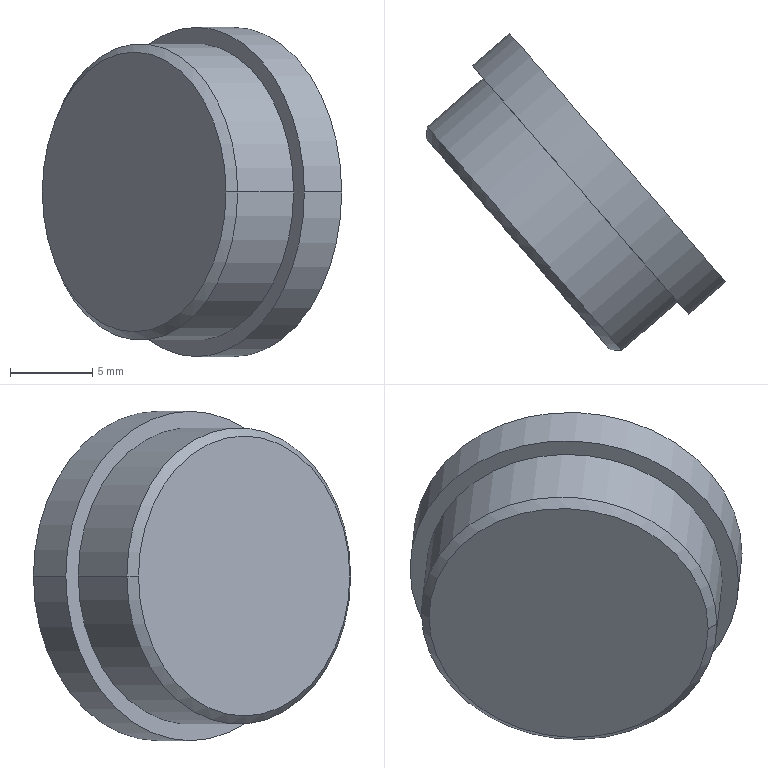Part | SolidWorks | features Chamfer 1, Revolution 1 | 1 solid | 9 faces | box 18.175 x 19.26 x 20 mm | volume 2208 mm3 | cylinder 4 | plane 3 | cone 2 | commonest cylinder face diameters 18 x2 20 x2
STEP:
#1=CARTESIAN_POINT('',(1439.201,-61.47,0.));
#2=VERTEX_POINT('',#1);
#3=CARTESIAN_POINT('',(1428.048,-48.64,0.));
#4=VERTEX_POINT('',#3);
#5=CARTESIAN_POINT('',(1433.624,-55.055,0.));
#6=DIRECTION('',(-0.7547,-0.6561,0.));
#7=DIRECTION('',(0.6561,-0.7547,0.));
#8=AXIS2_PLACEMENT_3D('',#5,#6,#7);
#9=CIRCLE('',#8,8.5);
#10=EDGE_CURVE('',#2,#4,#9,.T.);
#11=ORIENTED_EDGE('',*,*,#10,.F.);
#12=CARTESIAN_POINT('',(1439.906,-61.519,0.));
#13=VERTEX_POINT('',#12);
#14=CARTESIAN_POINT('',(1439.906,-61.519,0.));
#15=DIRECTION('',(0.9976,-0.06976,0.));
#16=VECTOR('',#15,1000.);
#17=LINE('',#14,#16);
#18=EDGE_CURVE('',#2,#13,#17,.T.);
#19=ORIENTED_EDGE('',*,*,#18,.T.);
#20=CARTESIAN_POINT('',(1428.097,-47.934,0.));
#21=VERTEX_POINT('',#20);
#22=CARTESIAN_POINT('',(1434.002,-54.727,0.));
#23=DIRECTION('',(0.7547,0.6561,0.));
#24=DIRECTION('',(0.6561,-0.7547,0.));
#25=AXIS2_PLACEMENT_3D('',#22,#23,#24);
#26=CIRCLE('',#25,9.);
#27=EDGE_CURVE('',#21,#13,#26,.T.);
#28=ORIENTED_EDGE('',*,*,#27,.F.);
#29=CARTESIAN_POINT('',(1428.097,-47.934,0.));
#30=DIRECTION('',(0.06976,0.9976,0.));
#31=VECTOR('',#30,1000.);
#32=LINE('',#29,#31);
#33=EDGE_CURVE('',#4,#21,#32,.T.);
#34=ORIENTED_EDGE('',*,*,#33,.F.);
#35=EDGE_LOOP('',(#11,#19,#28,#34));
#36=FACE_OUTER_BOUND('',#35,.T.);
#37=CARTESIAN_POINT('',(1434.002,-54.727,0.));
#38=DIRECTION('',(0.7547,0.6561,0.));
#39=DIRECTION('',(-0.6561,0.7547,0.));
#40=AXIS2_PLACEMENT_3D('',#37,#38,#39);
#41=CONICAL_SURFACE('',#40,9.,0.7854);
#42=ADVANCED_FACE('',(#36),#41,.T.);
#43=CARTESIAN_POINT('',(1430.837,-44.227,0.));
#44=VERTEX_POINT('',#43);
#45=CARTESIAN_POINT('',(1443.958,-59.322,0.));
#46=VERTEX_POINT('',#45);
#47=CARTESIAN_POINT('',(1437.398,-51.775,0.));
#48=DIRECTION('',(0.7547,0.6561,0.));
#49=DIRECTION('',(-0.6561,0.7547,0.));
#50=AXIS2_PLACEMENT_3D('',#47,#48,#49);
#51=CIRCLE('',#50,10.);
#52=EDGE_CURVE('',#44,#46,#51,.T.);
#53=ORIENTED_EDGE('',*,*,#52,.T.);
#54=CARTESIAN_POINT('',(1446.223,-57.354,0.));
#55=VERTEX_POINT('',#54);
#56=CARTESIAN_POINT('',(1446.223,-57.354,0.));
#57=DIRECTION('',(0.7547,0.6561,0.));
#58=VECTOR('',#57,1000.);
#59=LINE('',#56,#58);
#60=EDGE_CURVE('',#46,#55,#59,.T.);
#61=ORIENTED_EDGE('',*,*,#60,.T.);
#62=CARTESIAN_POINT('',(1433.101,-42.259,0.));
#63=VERTEX_POINT('',#62);
#64=CARTESIAN_POINT('',(1439.662,-49.806,0.));
#65=DIRECTION('',(0.7547,0.6561,0.));
#66=DIRECTION('',(-0.6561,0.7547,0.));
#67=AXIS2_PLACEMENT_3D('',#64,#65,#66);
#68=CIRCLE('',#67,10.);
#69=EDGE_CURVE('',#63,#55,#68,.T.);
#70=ORIENTED_EDGE('',*,*,#69,.F.);
#71=CARTESIAN_POINT('',(1433.101,-42.259,0.));
#72=DIRECTION('',(0.7547,0.6561,0.));
#73=VECTOR('',#72,1000.);
#74=LINE('',#71,#73);
#75=EDGE_CURVE('',#44,#63,#74,.T.);
#76=ORIENTED_EDGE('',*,*,#75,.F.);
#77=EDGE_LOOP('',(#53,#61,#70,#76));
#78=FACE_OUTER_BOUND('',#77,.T.);
#79=CARTESIAN_POINT('',(1439.662,-49.806,0.));
#80=DIRECTION('',(0.7547,0.6561,0.));
#81=DIRECTION('',(-0.6561,0.7547,0.));
#82=AXIS2_PLACEMENT_3D('',#79,#80,#81);
#83=CYLINDRICAL_SURFACE('',#82,10.);
#84=ADVANCED_FACE('',(#78),#83,.T.);
#85=ORIENTED_EDGE('',*,*,#27,.T.);
#86=CARTESIAN_POINT('',(1443.302,-58.567,0.));
#87=VERTEX_POINT('',#86);
#88=CARTESIAN_POINT('',(1445.566,-56.599,0.));
#89=DIRECTION('',(0.7547,0.6561,0.));
#90=VECTOR('',#89,1000.);
#91=LINE('',#88,#90);
#92=EDGE_CURVE('',#13,#87,#91,.T.);
#93=ORIENTED_EDGE('',*,*,#92,.T.);
#94=CARTESIAN_POINT('',(1431.493,-44.982,0.));
#95=VERTEX_POINT('',#94);
#96=CARTESIAN_POINT('',(1437.398,-51.775,0.));
#97=DIRECTION('',(0.7547,0.6561,0.));
#98=DIRECTION('',(-0.6561,0.7547,0.));
#99=AXIS2_PLACEMENT_3D('',#96,#97,#98);
#100=CIRCLE('',#99,9.);
#101=EDGE_CURVE('',#95,#87,#100,.T.);
#102=ORIENTED_EDGE('',*,*,#101,.F.);
#103=CARTESIAN_POINT('',(1433.757,-43.014,0.));
#104=DIRECTION('',(0.7547,0.6561,0.));
#105=VECTOR('',#104,1000.);
#106=LINE('',#103,#105);
#107=EDGE_CURVE('',#21,#95,#106,.T.);
#108=ORIENTED_EDGE('',*,*,#107,.F.);
#109=EDGE_LOOP('',(#85,#93,#102,#108));
#110=FACE_OUTER_BOUND('',#109,.T.);
#111=CARTESIAN_POINT('',(1439.662,-49.806,0.));
#112=DIRECTION('',(0.7547,0.6561,0.));
#113=DIRECTION('',(-0.6561,0.7547,0.));
#114=AXIS2_PLACEMENT_3D('',#111,#112,#113);
#115=CYLINDRICAL_SURFACE('',#114,9.);
#116=ADVANCED_FACE('',(#110),#115,.T.);
#117=ORIENTED_EDGE('',*,*,#92,.F.);
#118=CARTESIAN_POINT('',(1434.002,-54.727,0.));
#119=DIRECTION('',(0.7547,0.6561,0.));
#120=DIRECTION('',(0.6561,-0.7547,0.));
#121=AXIS2_PLACEMENT_3D('',#118,#119,#120);
#122=CIRCLE('',#121,9.);
#123=EDGE_CURVE('',#13,#21,#122,.T.);
#124=ORIENTED_EDGE('',*,*,#123,.T.);
#125=ORIENTED_EDGE('',*,*,#107,.T.);
#126=CARTESIAN_POINT('',(1437.398,-51.775,0.));
#127=DIRECTION('',(0.7547,0.6561,0.));
#128=DIRECTION('',(-0.6561,0.7547,0.));
#129=AXIS2_PLACEMENT_3D('',#126,#127,#128);
#130=CIRCLE('',#129,9.);
#131=EDGE_CURVE('',#87,#95,#130,.T.);
#132=ORIENTED_EDGE('',*,*,#131,.F.);
#133=EDGE_LOOP('',(#117,#124,#125,#132));
#134=FACE_OUTER_BOUND('',#133,.T.);
#135=CARTESIAN_POINT('',(1439.662,-49.806,0.));
#136=DIRECTION('',(0.7547,0.6561,0.));
#137=DIRECTION('',(-0.6561,0.7547,0.));
#138=AXIS2_PLACEMENT_3D('',#135,#136,#137);
#139=CYLINDRICAL_SURFACE('',#138,9.);
#140=ADVANCED_FACE('',(#134),#139,.T.);
#141=CARTESIAN_POINT('',(1433.624,-55.055,0.));
#142=DIRECTION('',(-0.7547,-0.6561,0.));
#143=DIRECTION('',(0.6561,-0.7547,0.));
#144=AXIS2_PLACEMENT_3D('',#141,#142,#143);
#145=CIRCLE('',#144,8.5);
#146=EDGE_CURVE('',#4,#2,#145,.T.);
#147=ORIENTED_EDGE('',*,*,#146,.T.);
#148=ORIENTED_EDGE('',*,*,#10,.T.);
#149=EDGE_LOOP('',(#147,#148));
#150=FACE_OUTER_BOUND('',#149,.T.);
#151=CARTESIAN_POINT('',(1427.72,-48.262,0.));
#152=DIRECTION('',(-0.7547,-0.6561,0.));
#153=DIRECTION('',(0.6561,-0.7547,0.));
#154=AXIS2_PLACEMENT_3D('',#151,#152,#153);
#155=PLANE('',#154);
#156=ADVANCED_FACE('',(#150),#155,.T.);
#157=ORIENTED_EDGE('',*,*,#69,.T.);
#158=CARTESIAN_POINT('',(1439.662,-49.806,0.));
#159=DIRECTION('',(0.7547,0.6561,0.));
#160=DIRECTION('',(-0.6561,0.7547,0.));
#161=AXIS2_PLACEMENT_3D('',#158,#159,#160);
#162=CIRCLE('',#161,10.);
#163=EDGE_CURVE('',#55,#63,#162,.T.);
#164=ORIENTED_EDGE('',*,*,#163,.T.);
#165=EDGE_LOOP('',(#157,#164));
#166=FACE_OUTER_BOUND('',#165,.T.);
#167=CARTESIAN_POINT('',(1433.101,-42.259,0.));
#168=DIRECTION('',(0.7547,0.6561,0.));
#169=DIRECTION('',(-0.6561,0.7547,0.));
#170=AXIS2_PLACEMENT_3D('',#167,#168,#169);
#171=PLANE('',#170);
#172=ADVANCED_FACE('',(#166),#171,.T.);
#173=ORIENTED_EDGE('',*,*,#60,.F.);
#174=CARTESIAN_POINT('',(1437.398,-51.775,0.));
#175=DIRECTION('',(0.7547,0.6561,0.));
#176=DIRECTION('',(-0.6561,0.7547,0.));
#177=AXIS2_PLACEMENT_3D('',#174,#175,#176);
#178=CIRCLE('',#177,10.);
#179=EDGE_CURVE('',#46,#44,#178,.T.);
#180=ORIENTED_EDGE('',*,*,#179,.T.);
#181=ORIENTED_EDGE('',*,*,#75,.T.);
#182=ORIENTED_EDGE('',*,*,#163,.F.);
#183=EDGE_LOOP('',(#173,#180,#181,#182));
#184=FACE_OUTER_BOUND('',#183,.T.);
#185=CARTESIAN_POINT('',(1439.662,-49.806,0.));
#186=DIRECTION('',(0.7547,0.6561,0.));
#187=DIRECTION('',(-0.6561,0.7547,0.));
#188=AXIS2_PLACEMENT_3D('',#185,#186,#187);
#189=CYLINDRICAL_SURFACE('',#188,10.);
#190=ADVANCED_FACE('',(#184),#189,.T.);
#191=ORIENTED_EDGE('',*,*,#101,.T.);
#192=ORIENTED_EDGE('',*,*,#131,.T.);
#193=EDGE_LOOP('',(#191,#192));
#194=FACE_BOUND('',#193,.T.);
#195=ORIENTED_EDGE('',*,*,#52,.F.);
#196=ORIENTED_EDGE('',*,*,#179,.F.);
#197=EDGE_LOOP('',(#195,#196));
#198=FACE_OUTER_BOUND('',#197,.T.);
#199=CARTESIAN_POINT('',(1431.493,-44.982,0.));
#200=DIRECTION('',(-0.7547,-0.6561,0.));
#201=DIRECTION('',(0.6561,-0.7547,0.));
#202=AXIS2_PLACEMENT_3D('',#199,#200,#201);
#203=PLANE('',#202);
#204=ADVANCED_FACE('',(#194,#198),#203,.T.);
#205=ORIENTED_EDGE('',*,*,#18,.F.);
#206=ORIENTED_EDGE('',*,*,#146,.F.);
#207=ORIENTED_EDGE('',*,*,#33,.T.);
#208=ORIENTED_EDGE('',*,*,#123,.F.);
#209=EDGE_LOOP('',(#205,#206,#207,#208));
#210=FACE_OUTER_BOUND('',#209,.T.);
#211=CARTESIAN_POINT('',(1434.002,-54.727,0.));
#212=DIRECTION('',(0.7547,0.6561,0.));
#213=DIRECTION('',(-0.6561,0.7547,0.));
#214=AXIS2_PLACEMENT_3D('',#211,#212,#213);
#215=CONICAL_SURFACE('',#214,9.,0.7854);
#216=ADVANCED_FACE('',(#210),#215,.T.);
#217=CLOSED_SHELL('',(#42,#84,#116,#140,#156,#172,#190,#204,#216));
#218=MANIFOLD_SOLID_BREP('',#217);
#219=CARTESIAN_POINT('',(0.,0.,0.));
#220=DIRECTION('',(0.,0.,1.));
#221=DIRECTION('',(1.,0.,0.));
#222=AXIS2_PLACEMENT_3D('',#219,#220,#221);
#223=(LENGTH_UNIT()NAMED_UNIT(*)SI_UNIT(.MILLI.,.METRE.));
#224=UNCERTAINTY_MEASURE_WITH_UNIT(LENGTH_MEASURE(0.00001),#223,'','');
#225=(NAMED_UNIT(*)PLANE_ANGLE_UNIT()SI_UNIT($,.RADIAN.));
#226=(NAMED_UNIT(*)SI_UNIT($,.STERADIAN.)SOLID_ANGLE_UNIT());
#227=(GEOMETRIC_REPRESENTATION_CONTEXT(3)GLOBAL_UNCERTAINTY_ASSIGNED_CONTEXT((#224))GLOBAL_UNIT_ASSIGNED_CONTEXT((#223,#225,#226))REPRESENTATION_CONTEXT('',''));
#228=ADVANCED_BREP_SHAPE_REPRESENTATION('',(#218,#222),#227);